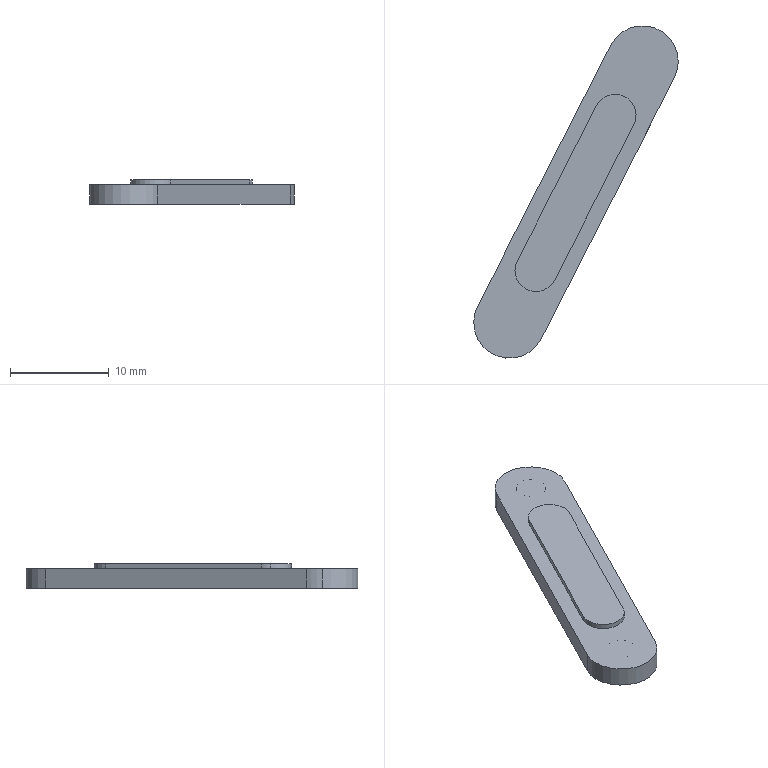Part | SolidWorks | features ICE 3, Extrusion 1 | 1 solid | 19 faces | box 20.758 x 33.747 x 2.5 mm | volume 532.773 mm3 | cylinder 10 | plane 9 | commonest cylinder face diameters 3 x4 4.262 x3 7.265 x3
STEP:
#1=CARTESIAN_POINT('',(1.405,14.797,1.5));
#2=VERTEX_POINT('',#1);
#3=CARTESIAN_POINT('',(5.435,13.83,1.5));
#4=VERTEX_POINT('',#3);
#5=CARTESIAN_POINT('',(3.536,14.797,1.5));
#6=DIRECTION('',(0.,0.,1.));
#7=DIRECTION('',(1.,0.,0.));
#8=AXIS2_PLACEMENT_3D('',#5,#6,#7);
#9=CIRCLE('',#8,2.131);
#10=EDGE_CURVE('',#2,#4,#9,.T.);
#11=ORIENTED_EDGE('',*,*,#10,.F.);
#12=CARTESIAN_POINT('',(1.405,14.797,1.));
#13=VERTEX_POINT('',#12);
#14=CARTESIAN_POINT('',(1.405,14.797,1.5));
#15=DIRECTION('',(0.,0.,-1.));
#16=VECTOR('',#15,1000.);
#17=LINE('',#14,#16);
#18=EDGE_CURVE('',#2,#13,#17,.T.);
#19=ORIENTED_EDGE('',*,*,#18,.T.);
#20=CARTESIAN_POINT('',(5.435,13.83,1.));
#21=VERTEX_POINT('',#20);
#22=CARTESIAN_POINT('',(3.536,14.797,1.));
#23=DIRECTION('',(0.,0.,-1.));
#24=DIRECTION('',(1.,0.,0.));
#25=AXIS2_PLACEMENT_3D('',#22,#23,#24);
#26=CIRCLE('',#25,2.131);
#27=EDGE_CURVE('',#21,#13,#26,.T.);
#28=ORIENTED_EDGE('',*,*,#27,.F.);
#29=CARTESIAN_POINT('',(5.435,13.83,1.5));
#30=DIRECTION('',(0.,0.,-1.));
#31=VECTOR('',#30,1000.);
#32=LINE('',#29,#31);
#33=EDGE_CURVE('',#4,#21,#32,.T.);
#34=ORIENTED_EDGE('',*,*,#33,.F.);
#35=EDGE_LOOP('',(#11,#19,#28,#34));
#36=FACE_OUTER_BOUND('',#35,.T.);
#37=CARTESIAN_POINT('',(3.536,14.797,1.5));
#38=DIRECTION('',(0.,0.,-1.));
#39=DIRECTION('',(-1.,0.,0.));
#40=AXIS2_PLACEMENT_3D('',#37,#38,#39);
#41=CYLINDRICAL_SURFACE('',#40,2.131);
#42=ADVANCED_FACE('',(#36),#41,.T.);
#43=CARTESIAN_POINT('',(-2.775,9.541,1.));
#44=VERTEX_POINT('',#43);
#45=CARTESIAN_POINT('',(4.094,7.891,1.));
#46=VERTEX_POINT('',#45);
#47=CARTESIAN_POINT('',(0.8578,9.541,1.));
#48=DIRECTION('',(0.,0.,1.));
#49=DIRECTION('',(1.,0.,0.));
#50=AXIS2_PLACEMENT_3D('',#47,#48,#49);
#51=CIRCLE('',#50,3.633);
#52=EDGE_CURVE('',#44,#46,#51,.T.);
#53=ORIENTED_EDGE('',*,*,#52,.F.);
#54=CARTESIAN_POINT('',(-2.775,9.541,-1.));
#55=VERTEX_POINT('',#54);
#56=CARTESIAN_POINT('',(-2.775,9.541,1.));
#57=DIRECTION('',(0.,0.,-1.));
#58=VECTOR('',#57,1000.);
#59=LINE('',#56,#58);
#60=EDGE_CURVE('',#44,#55,#59,.T.);
#61=ORIENTED_EDGE('',*,*,#60,.T.);
#62=CARTESIAN_POINT('',(4.094,7.891,-1.));
#63=VERTEX_POINT('',#62);
#64=CARTESIAN_POINT('',(0.8578,9.541,-1.));
#65=DIRECTION('',(0.,0.,1.));
#66=DIRECTION('',(1.,0.,0.));
#67=AXIS2_PLACEMENT_3D('',#64,#65,#66);
#68=CIRCLE('',#67,3.633);
#69=EDGE_CURVE('',#55,#63,#68,.T.);
#70=ORIENTED_EDGE('',*,*,#69,.T.);
#71=CARTESIAN_POINT('',(4.094,7.891,1.));
#72=DIRECTION('',(0.,0.,-1.));
#73=VECTOR('',#72,1000.);
#74=LINE('',#71,#73);
#75=EDGE_CURVE('',#46,#63,#74,.T.);
#76=ORIENTED_EDGE('',*,*,#75,.F.);
#77=EDGE_LOOP('',(#53,#61,#70,#76));
#78=FACE_OUTER_BOUND('',#77,.T.);
#79=CARTESIAN_POINT('',(0.8578,9.541,1.));
#80=DIRECTION('',(0.,0.,-1.));
#81=DIRECTION('',(-1.,0.,0.));
#82=AXIS2_PLACEMENT_3D('',#79,#80,#81);
#83=CYLINDRICAL_SURFACE('',#82,3.633);
#84=ADVANCED_FACE('',(#78),#83,.T.);
#85=CARTESIAN_POINT('',(-0.6422,9.541,0.9));
#86=VERTEX_POINT('',#85);
#87=CARTESIAN_POINT('',(2.358,9.541,0.9));
#88=VERTEX_POINT('',#87);
#89=CARTESIAN_POINT('',(0.8578,9.541,0.9));
#90=DIRECTION('',(0.,0.,1.));
#91=DIRECTION('',(1.,0.,0.));
#92=AXIS2_PLACEMENT_3D('',#89,#90,#91);
#93=CIRCLE('',#92,1.5);
#94=EDGE_CURVE('',#86,#88,#93,.T.);
#95=ORIENTED_EDGE('',*,*,#94,.T.);
#96=CARTESIAN_POINT('',(2.358,9.541,-1.));
#97=VERTEX_POINT('',#96);
#98=CARTESIAN_POINT('',(2.358,9.541,1.));
#99=DIRECTION('',(0.,0.,-1.));
#100=VECTOR('',#99,1000.);
#101=LINE('',#98,#100);
#102=EDGE_CURVE('',#88,#97,#101,.T.);
#103=ORIENTED_EDGE('',*,*,#102,.T.);
#104=CARTESIAN_POINT('',(-0.6422,9.541,-1.));
#105=VERTEX_POINT('',#104);
#106=CARTESIAN_POINT('',(0.8578,9.541,-1.));
#107=DIRECTION('',(0.,0.,1.));
#108=DIRECTION('',(1.,0.,0.));
#109=AXIS2_PLACEMENT_3D('',#106,#107,#108);
#110=CIRCLE('',#109,1.5);
#111=EDGE_CURVE('',#105,#97,#110,.T.);
#112=ORIENTED_EDGE('',*,*,#111,.F.);
#113=CARTESIAN_POINT('',(-0.6422,9.541,1.));
#114=DIRECTION('',(0.,0.,-1.));
#115=VECTOR('',#114,1000.);
#116=LINE('',#113,#115);
#117=EDGE_CURVE('',#86,#105,#116,.T.);
#118=ORIENTED_EDGE('',*,*,#117,.F.);
#119=EDGE_LOOP('',(#95,#103,#112,#118));
#120=FACE_OUTER_BOUND('',#119,.T.);
#121=CARTESIAN_POINT('',(0.8578,9.541,1.));
#122=DIRECTION('',(0.,0.,-1.));
#123=DIRECTION('',(-1.,0.,0.));
#124=AXIS2_PLACEMENT_3D('',#121,#122,#123);
#125=CYLINDRICAL_SURFACE('',#124,1.5);
#126=ADVANCED_FACE('',(#120),#125,.F.);
#127=CARTESIAN_POINT('',(12.851,36.022,0.9));
#128=VERTEX_POINT('',#127);
#129=CARTESIAN_POINT('',(15.851,36.022,0.9));
#130=VERTEX_POINT('',#129);
#131=CARTESIAN_POINT('',(14.351,36.022,0.9));
#132=DIRECTION('',(0.,0.,1.));
#133=DIRECTION('',(1.,0.,0.));
#134=AXIS2_PLACEMENT_3D('',#131,#132,#133);
#135=CIRCLE('',#134,1.5);
#136=EDGE_CURVE('',#128,#130,#135,.T.);
#137=ORIENTED_EDGE('',*,*,#136,.T.);
#138=CARTESIAN_POINT('',(15.851,36.022,-1.));
#139=VERTEX_POINT('',#138);
#140=CARTESIAN_POINT('',(15.851,36.022,1.));
#141=DIRECTION('',(0.,0.,-1.));
#142=VECTOR('',#141,1000.);
#143=LINE('',#140,#142);
#144=EDGE_CURVE('',#130,#139,#143,.T.);
#145=ORIENTED_EDGE('',*,*,#144,.T.);
#146=CARTESIAN_POINT('',(12.851,36.022,-1.));
#147=VERTEX_POINT('',#146);
#148=CARTESIAN_POINT('',(14.351,36.022,-1.));
#149=DIRECTION('',(0.,0.,1.));
#150=DIRECTION('',(1.,0.,0.));
#151=AXIS2_PLACEMENT_3D('',#148,#149,#150);
#152=CIRCLE('',#151,1.5);
#153=EDGE_CURVE('',#147,#139,#152,.T.);
#154=ORIENTED_EDGE('',*,*,#153,.F.);
#155=CARTESIAN_POINT('',(12.851,36.022,1.));
#156=DIRECTION('',(0.,0.,-1.));
#157=VECTOR('',#156,1000.);
#158=LINE('',#155,#157);
#159=EDGE_CURVE('',#128,#147,#158,.T.);
#160=ORIENTED_EDGE('',*,*,#159,.F.);
#161=EDGE_LOOP('',(#137,#145,#154,#160));
#162=FACE_OUTER_BOUND('',#161,.T.);
#163=CARTESIAN_POINT('',(14.351,36.022,1.));
#164=DIRECTION('',(0.,0.,-1.));
#165=DIRECTION('',(-1.,0.,0.));
#166=AXIS2_PLACEMENT_3D('',#163,#164,#165);
#167=CYLINDRICAL_SURFACE('',#166,1.5);
#168=ADVANCED_FACE('',(#162),#167,.F.);
#169=ORIENTED_EDGE('',*,*,#144,.F.);
#170=CARTESIAN_POINT('',(14.351,36.022,0.9));
#171=DIRECTION('',(0.,0.,1.));
#172=DIRECTION('',(1.,0.,0.));
#173=AXIS2_PLACEMENT_3D('',#170,#171,#172);
#174=CIRCLE('',#173,1.5);
#175=EDGE_CURVE('',#130,#128,#174,.T.);
#176=ORIENTED_EDGE('',*,*,#175,.T.);
#177=ORIENTED_EDGE('',*,*,#159,.T.);
#178=CARTESIAN_POINT('',(14.351,36.022,-1.));
#179=DIRECTION('',(0.,0.,1.));
#180=DIRECTION('',(1.,0.,0.));
#181=AXIS2_PLACEMENT_3D('',#178,#179,#180);
#182=CIRCLE('',#181,1.5);
#183=EDGE_CURVE('',#139,#147,#182,.T.);
#184=ORIENTED_EDGE('',*,*,#183,.F.);
#185=EDGE_LOOP('',(#169,#176,#177,#184));
#186=FACE_OUTER_BOUND('',#185,.T.);
#187=CARTESIAN_POINT('',(14.351,36.022,1.));
#188=DIRECTION('',(0.,0.,-1.));
#189=DIRECTION('',(-1.,0.,0.));
#190=AXIS2_PLACEMENT_3D('',#187,#188,#189);
#191=CYLINDRICAL_SURFACE('',#190,1.5);
#192=ADVANCED_FACE('',(#186),#191,.F.);
#193=ORIENTED_EDGE('',*,*,#102,.F.);
#194=CARTESIAN_POINT('',(0.8578,9.541,0.9));
#195=DIRECTION('',(0.,0.,1.));
#196=DIRECTION('',(1.,0.,0.));
#197=AXIS2_PLACEMENT_3D('',#194,#195,#196);
#198=CIRCLE('',#197,1.5);
#199=EDGE_CURVE('',#88,#86,#198,.T.);
#200=ORIENTED_EDGE('',*,*,#199,.T.);
#201=ORIENTED_EDGE('',*,*,#117,.T.);
#202=CARTESIAN_POINT('',(0.8578,9.541,-1.));
#203=DIRECTION('',(0.,0.,1.));
#204=DIRECTION('',(1.,0.,0.));
#205=AXIS2_PLACEMENT_3D('',#202,#203,#204);
#206=CIRCLE('',#205,1.5);
#207=EDGE_CURVE('',#97,#105,#206,.T.);
#208=ORIENTED_EDGE('',*,*,#207,.F.);
#209=EDGE_LOOP('',(#193,#200,#201,#208));
#210=FACE_OUTER_BOUND('',#209,.T.);
#211=CARTESIAN_POINT('',(0.8578,9.541,1.));
#212=DIRECTION('',(0.,0.,-1.));
#213=DIRECTION('',(-1.,0.,0.));
#214=AXIS2_PLACEMENT_3D('',#211,#212,#213);
#215=CYLINDRICAL_SURFACE('',#214,1.5);
#216=ADVANCED_FACE('',(#210),#215,.F.);
#217=CARTESIAN_POINT('',(17.588,34.373,1.));
#218=VERTEX_POINT('',#217);
#219=CARTESIAN_POINT('',(0.05832,-0.02971,1.));
#220=DIRECTION('',(0.454,0.891,0.));
#221=VECTOR('',#220,1000.);
#222=LINE('',#219,#221);
#223=EDGE_CURVE('',#46,#218,#222,.T.);
#224=ORIENTED_EDGE('',*,*,#223,.T.);
#225=CARTESIAN_POINT('',(11.114,37.671,1.));
#226=VERTEX_POINT('',#225);
#227=CARTESIAN_POINT('',(14.351,36.022,1.));
#228=DIRECTION('',(0.,0.,1.));
#229=DIRECTION('',(1.,0.,0.));
#230=AXIS2_PLACEMENT_3D('',#227,#228,#229);
#231=CIRCLE('',#230,3.633);
#232=EDGE_CURVE('',#218,#226,#231,.T.);
#233=ORIENTED_EDGE('',*,*,#232,.T.);
#234=CARTESIAN_POINT('',(-2.379,11.19,1.));
#235=VERTEX_POINT('',#234);
#236=CARTESIAN_POINT('',(-6.415,3.269,1.));
#237=DIRECTION('',(0.454,0.891,0.));
#238=VECTOR('',#237,1000.);
#239=LINE('',#236,#238);
#240=EDGE_CURVE('',#235,#226,#239,.T.);
#241=ORIENTED_EDGE('',*,*,#240,.F.);
#242=CARTESIAN_POINT('',(0.8578,9.541,1.));
#243=DIRECTION('',(0.,0.,1.));
#244=DIRECTION('',(1.,0.,0.));
#245=AXIS2_PLACEMENT_3D('',#242,#243,#244);
#246=CIRCLE('',#245,3.633);
#247=EDGE_CURVE('',#235,#44,#246,.T.);
#248=ORIENTED_EDGE('',*,*,#247,.T.);
#249=ORIENTED_EDGE('',*,*,#52,.T.);
#250=EDGE_LOOP('',(#224,#233,#241,#248,#249));
#251=FACE_OUTER_BOUND('',#250,.T.);
#252=CARTESIAN_POINT('',(13.474,29.607,1.));
#253=VERTEX_POINT('',#252);
#254=CARTESIAN_POINT('',(-1.28,0.652,1.));
#255=DIRECTION('',(-0.454,-0.891,0.));
#256=VECTOR('',#255,1000.);
#257=LINE('',#254,#256);
#258=EDGE_CURVE('',#253,#21,#257,.T.);
#259=ORIENTED_EDGE('',*,*,#258,.T.);
#260=ORIENTED_EDGE('',*,*,#27,.T.);
#261=CARTESIAN_POINT('',(1.637,15.764,1.));
#262=VERTEX_POINT('',#261);
#263=CARTESIAN_POINT('',(3.536,14.797,1.));
#264=DIRECTION('',(0.,0.,-1.));
#265=DIRECTION('',(1.,0.,0.));
#266=AXIS2_PLACEMENT_3D('',#263,#264,#265);
#267=CIRCLE('',#266,2.131);
#268=EDGE_CURVE('',#13,#262,#267,.T.);
#269=ORIENTED_EDGE('',*,*,#268,.T.);
#270=CARTESIAN_POINT('',(9.677,31.542,1.));
#271=VERTEX_POINT('',#270);
#272=CARTESIAN_POINT('',(-5.077,2.587,1.));
#273=DIRECTION('',(0.454,0.891,0.));
#274=VECTOR('',#273,1000.);
#275=LINE('',#272,#274);
#276=EDGE_CURVE('',#262,#271,#275,.T.);
#277=ORIENTED_EDGE('',*,*,#276,.T.);
#278=CARTESIAN_POINT('',(11.575,30.575,1.));
#279=DIRECTION('',(0.,0.,-1.));
#280=DIRECTION('',(1.,0.,0.));
#281=AXIS2_PLACEMENT_3D('',#278,#279,#280);
#282=CIRCLE('',#281,2.131);
#283=EDGE_CURVE('',#271,#253,#282,.T.);
#284=ORIENTED_EDGE('',*,*,#283,.T.);
#285=EDGE_LOOP('',(#259,#260,#269,#277,#284));
#286=FACE_BOUND('',#285,.T.);
#287=CARTESIAN_POINT('',(0.,0.,1.));
#288=DIRECTION('',(0.,0.,1.));
#289=DIRECTION('',(1.,0.,0.));
#290=AXIS2_PLACEMENT_3D('',#287,#288,#289);
#291=PLANE('',#290);
#292=ADVANCED_FACE('',(#251,#286),#291,.T.);
#293=CARTESIAN_POINT('',(17.588,34.373,-1.));
#294=VERTEX_POINT('',#293);
#295=CARTESIAN_POINT('',(0.05832,-0.02971,-1.));
#296=DIRECTION('',(0.454,0.891,0.));
#297=VECTOR('',#296,1000.);
#298=LINE('',#295,#297);
#299=EDGE_CURVE('',#63,#294,#298,.T.);
#300=ORIENTED_EDGE('',*,*,#299,.T.);
#301=CARTESIAN_POINT('',(17.588,34.373,1.));
#302=DIRECTION('',(0.,0.,-1.));
#303=VECTOR('',#302,1000.);
#304=LINE('',#301,#303);
#305=EDGE_CURVE('',#218,#294,#304,.T.);
#306=ORIENTED_EDGE('',*,*,#305,.F.);
#307=ORIENTED_EDGE('',*,*,#223,.F.);
#308=ORIENTED_EDGE('',*,*,#75,.T.);
#309=EDGE_LOOP('',(#300,#306,#307,#308));
#310=FACE_OUTER_BOUND('',#309,.T.);
#311=CARTESIAN_POINT('',(0.05832,-0.02971,1.));
#312=DIRECTION('',(-0.891,0.454,0.));
#313=DIRECTION('',(-0.454,-0.891,0.));
#314=AXIS2_PLACEMENT_3D('',#311,#312,#313);
#315=PLANE('',#314);
#316=ADVANCED_FACE('',(#310),#315,.F.);
#317=CARTESIAN_POINT('',(11.114,37.671,-1.));
#318=VERTEX_POINT('',#317);
#319=CARTESIAN_POINT('',(14.351,36.022,-1.));
#320=DIRECTION('',(0.,0.,1.));
#321=DIRECTION('',(1.,0.,0.));
#322=AXIS2_PLACEMENT_3D('',#319,#320,#321);
#323=CIRCLE('',#322,3.633);
#324=EDGE_CURVE('',#294,#318,#323,.T.);
#325=ORIENTED_EDGE('',*,*,#324,.T.);
#326=CARTESIAN_POINT('',(11.114,37.671,1.));
#327=DIRECTION('',(0.,0.,-1.));
#328=VECTOR('',#327,1000.);
#329=LINE('',#326,#328);
#330=EDGE_CURVE('',#226,#318,#329,.T.);
#331=ORIENTED_EDGE('',*,*,#330,.F.);
#332=ORIENTED_EDGE('',*,*,#232,.F.);
#333=ORIENTED_EDGE('',*,*,#305,.T.);
#334=EDGE_LOOP('',(#325,#331,#332,#333));
#335=FACE_OUTER_BOUND('',#334,.T.);
#336=CARTESIAN_POINT('',(14.351,36.022,1.));
#337=DIRECTION('',(0.,0.,-1.));
#338=DIRECTION('',(-1.,0.,0.));
#339=AXIS2_PLACEMENT_3D('',#336,#337,#338);
#340=CYLINDRICAL_SURFACE('',#339,3.633);
#341=ADVANCED_FACE('',(#335),#340,.T.);
#342=CARTESIAN_POINT('',(-2.379,11.19,-1.));
#343=VERTEX_POINT('',#342);
#344=CARTESIAN_POINT('',(-6.415,3.269,-1.));
#345=DIRECTION('',(0.454,0.891,0.));
#346=VECTOR('',#345,1000.);
#347=LINE('',#344,#346);
#348=EDGE_CURVE('',#343,#318,#347,.T.);
#349=ORIENTED_EDGE('',*,*,#348,.F.);
#350=CARTESIAN_POINT('',(-2.379,11.19,1.));
#351=DIRECTION('',(0.,0.,-1.));
#352=VECTOR('',#351,1000.);
#353=LINE('',#350,#352);
#354=EDGE_CURVE('',#235,#343,#353,.T.);
#355=ORIENTED_EDGE('',*,*,#354,.F.);
#356=ORIENTED_EDGE('',*,*,#240,.T.);
#357=ORIENTED_EDGE('',*,*,#330,.T.);
#358=EDGE_LOOP('',(#349,#355,#356,#357));
#359=FACE_OUTER_BOUND('',#358,.T.);
#360=CARTESIAN_POINT('',(-6.415,3.269,1.));
#361=DIRECTION('',(-0.891,0.454,0.));
#362=DIRECTION('',(-0.454,-0.891,0.));
#363=AXIS2_PLACEMENT_3D('',#360,#361,#362);
#364=PLANE('',#363);
#365=ADVANCED_FACE('',(#359),#364,.T.);
#366=ORIENTED_EDGE('',*,*,#60,.F.);
#367=ORIENTED_EDGE('',*,*,#247,.F.);
#368=ORIENTED_EDGE('',*,*,#354,.T.);
#369=CARTESIAN_POINT('',(0.8578,9.541,-1.));
#370=DIRECTION('',(0.,0.,1.));
#371=DIRECTION('',(1.,0.,0.));
#372=AXIS2_PLACEMENT_3D('',#369,#370,#371);
#373=CIRCLE('',#372,3.633);
#374=EDGE_CURVE('',#343,#55,#373,.T.);
#375=ORIENTED_EDGE('',*,*,#374,.T.);
#376=EDGE_LOOP('',(#366,#367,#368,#375));
#377=FACE_OUTER_BOUND('',#376,.T.);
#378=CARTESIAN_POINT('',(0.8578,9.541,1.));
#379=DIRECTION('',(0.,0.,-1.));
#380=DIRECTION('',(-1.,0.,0.));
#381=AXIS2_PLACEMENT_3D('',#378,#379,#380);
#382=CYLINDRICAL_SURFACE('',#381,3.633);
#383=ADVANCED_FACE('',(#377),#382,.T.);
#384=ORIENTED_EDGE('',*,*,#153,.T.);
#385=ORIENTED_EDGE('',*,*,#183,.T.);
#386=EDGE_LOOP('',(#384,#385));
#387=FACE_BOUND('',#386,.T.);
#388=ORIENTED_EDGE('',*,*,#111,.T.);
#389=ORIENTED_EDGE('',*,*,#207,.T.);
#390=EDGE_LOOP('',(#388,#389));
#391=FACE_BOUND('',#390,.T.);
#392=ORIENTED_EDGE('',*,*,#299,.F.);
#393=ORIENTED_EDGE('',*,*,#69,.F.);
#394=ORIENTED_EDGE('',*,*,#374,.F.);
#395=ORIENTED_EDGE('',*,*,#348,.T.);
#396=ORIENTED_EDGE('',*,*,#324,.F.);
#397=EDGE_LOOP('',(#392,#393,#394,#395,#396));
#398=FACE_OUTER_BOUND('',#397,.T.);
#399=CARTESIAN_POINT('',(0.,0.,-1.));
#400=DIRECTION('',(0.,0.,1.));
#401=DIRECTION('',(1.,0.,0.));
#402=AXIS2_PLACEMENT_3D('',#399,#400,#401);
#403=PLANE('',#402);
#404=ADVANCED_FACE('',(#387,#391,#398),#403,.F.);
#405=ORIENTED_EDGE('',*,*,#18,.F.);
#406=CARTESIAN_POINT('',(1.637,15.764,1.5));
#407=VERTEX_POINT('',#406);
#408=CARTESIAN_POINT('',(3.536,14.797,1.5));
#409=DIRECTION('',(0.,0.,1.));
#410=DIRECTION('',(1.,0.,0.));
#411=AXIS2_PLACEMENT_3D('',#408,#409,#410);
#412=CIRCLE('',#411,2.131);
#413=EDGE_CURVE('',#407,#2,#412,.T.);
#414=ORIENTED_EDGE('',*,*,#413,.F.);
#415=CARTESIAN_POINT('',(1.637,15.764,1.5));
#416=DIRECTION('',(0.,0.,-1.));
#417=VECTOR('',#416,1000.);
#418=LINE('',#415,#417);
#419=EDGE_CURVE('',#407,#262,#418,.T.);
#420=ORIENTED_EDGE('',*,*,#419,.T.);
#421=ORIENTED_EDGE('',*,*,#268,.F.);
#422=EDGE_LOOP('',(#405,#414,#420,#421));
#423=FACE_OUTER_BOUND('',#422,.T.);
#424=CARTESIAN_POINT('',(3.536,14.797,1.5));
#425=DIRECTION('',(0.,0.,-1.));
#426=DIRECTION('',(-1.,0.,0.));
#427=AXIS2_PLACEMENT_3D('',#424,#425,#426);
#428=CYLINDRICAL_SURFACE('',#427,2.131);
#429=ADVANCED_FACE('',(#423),#428,.T.);
#430=ORIENTED_EDGE('',*,*,#258,.F.);
#431=CARTESIAN_POINT('',(13.474,29.607,1.5));
#432=VERTEX_POINT('',#431);
#433=CARTESIAN_POINT('',(13.474,29.607,1.5));
#434=DIRECTION('',(0.,0.,-1.));
#435=VECTOR('',#434,1000.);
#436=LINE('',#433,#435);
#437=EDGE_CURVE('',#432,#253,#436,.T.);
#438=ORIENTED_EDGE('',*,*,#437,.F.);
#439=CARTESIAN_POINT('',(5.435,13.83,1.5));
#440=DIRECTION('',(0.454,0.891,0.));
#441=VECTOR('',#440,1000.);
#442=LINE('',#439,#441);
#443=EDGE_CURVE('',#4,#432,#442,.T.);
#444=ORIENTED_EDGE('',*,*,#443,.F.);
#445=ORIENTED_EDGE('',*,*,#33,.T.);
#446=EDGE_LOOP('',(#430,#438,#444,#445));
#447=FACE_OUTER_BOUND('',#446,.T.);
#448=CARTESIAN_POINT('',(5.435,13.83,1.5));
#449=DIRECTION('',(-0.891,0.454,0.));
#450=DIRECTION('',(-0.454,-0.891,0.));
#451=AXIS2_PLACEMENT_3D('',#448,#449,#450);
#452=PLANE('',#451);
#453=ADVANCED_FACE('',(#447),#452,.F.);
#454=ORIENTED_EDGE('',*,*,#283,.F.);
#455=CARTESIAN_POINT('',(9.677,31.542,1.5));
#456=VERTEX_POINT('',#455);
#457=CARTESIAN_POINT('',(9.677,31.542,1.5));
#458=DIRECTION('',(0.,0.,-1.));
#459=VECTOR('',#458,1000.);
#460=LINE('',#457,#459);
#461=EDGE_CURVE('',#456,#271,#460,.T.);
#462=ORIENTED_EDGE('',*,*,#461,.F.);
#463=CARTESIAN_POINT('',(11.575,30.575,1.5));
#464=DIRECTION('',(0.,0.,1.));
#465=DIRECTION('',(1.,0.,0.));
#466=AXIS2_PLACEMENT_3D('',#463,#464,#465);
#467=CIRCLE('',#466,2.131);
#468=EDGE_CURVE('',#432,#456,#467,.T.);
#469=ORIENTED_EDGE('',*,*,#468,.F.);
#470=ORIENTED_EDGE('',*,*,#437,.T.);
#471=EDGE_LOOP('',(#454,#462,#469,#470));
#472=FACE_OUTER_BOUND('',#471,.T.);
#473=CARTESIAN_POINT('',(11.575,30.575,1.5));
#474=DIRECTION('',(0.,0.,-1.));
#475=DIRECTION('',(-1.,0.,0.));
#476=AXIS2_PLACEMENT_3D('',#473,#474,#475);
#477=CYLINDRICAL_SURFACE('',#476,2.131);
#478=ADVANCED_FACE('',(#472),#477,.T.);
#479=ORIENTED_EDGE('',*,*,#276,.F.);
#480=ORIENTED_EDGE('',*,*,#419,.F.);
#481=CARTESIAN_POINT('',(1.637,15.764,1.5));
#482=DIRECTION('',(-0.454,-0.891,0.));
#483=VECTOR('',#482,1000.);
#484=LINE('',#481,#483);
#485=EDGE_CURVE('',#456,#407,#484,.T.);
#486=ORIENTED_EDGE('',*,*,#485,.F.);
#487=ORIENTED_EDGE('',*,*,#461,.T.);
#488=EDGE_LOOP('',(#479,#480,#486,#487));
#489=FACE_OUTER_BOUND('',#488,.T.);
#490=CARTESIAN_POINT('',(1.637,15.764,1.5));
#491=DIRECTION('',(0.891,-0.454,0.));
#492=DIRECTION('',(0.454,0.891,0.));
#493=AXIS2_PLACEMENT_3D('',#490,#491,#492);
#494=PLANE('',#493);
#495=ADVANCED_FACE('',(#489),#494,.F.);
#496=ORIENTED_EDGE('',*,*,#413,.T.);
#497=ORIENTED_EDGE('',*,*,#10,.T.);
#498=ORIENTED_EDGE('',*,*,#443,.T.);
#499=ORIENTED_EDGE('',*,*,#468,.T.);
#500=ORIENTED_EDGE('',*,*,#485,.T.);
#501=EDGE_LOOP('',(#496,#497,#498,#499,#500));
#502=FACE_OUTER_BOUND('',#501,.T.);
#503=CARTESIAN_POINT('',(3.536,14.797,1.5));
#504=DIRECTION('',(0.,0.,1.));
#505=DIRECTION('',(1.,0.,0.));
#506=AXIS2_PLACEMENT_3D('',#503,#504,#505);
#507=PLANE('',#506);
#508=ADVANCED_FACE('',(#502),#507,.T.);
#509=ORIENTED_EDGE('',*,*,#94,.F.);
#510=ORIENTED_EDGE('',*,*,#199,.F.);
#511=EDGE_LOOP('',(#509,#510));
#512=FACE_OUTER_BOUND('',#511,.T.);
#513=CARTESIAN_POINT('',(0.8578,9.541,0.9));
#514=DIRECTION('',(0.,0.,1.));
#515=DIRECTION('',(1.,0.,0.));
#516=AXIS2_PLACEMENT_3D('',#513,#514,#515);
#517=PLANE('',#516);
#518=ADVANCED_FACE('',(#512),#517,.F.);
#519=ORIENTED_EDGE('',*,*,#136,.F.);
#520=ORIENTED_EDGE('',*,*,#175,.F.);
#521=EDGE_LOOP('',(#519,#520));
#522=FACE_OUTER_BOUND('',#521,.T.);
#523=CARTESIAN_POINT('',(14.351,36.022,0.9));
#524=DIRECTION('',(0.,0.,1.));
#525=DIRECTION('',(1.,0.,0.));
#526=AXIS2_PLACEMENT_3D('',#523,#524,#525);
#527=PLANE('',#526);
#528=ADVANCED_FACE('',(#522),#527,.F.);
#529=CLOSED_SHELL('',(#42,#84,#126,#168,#192,#216,#292,#316,#341,#365,#383,#404,#429,#453,#478,#495,#508,#518,#528));
#530=MANIFOLD_SOLID_BREP('',#529);
#531=CARTESIAN_POINT('',(0.,0.,0.));
#532=DIRECTION('',(0.,0.,1.));
#533=DIRECTION('',(1.,0.,0.));
#534=AXIS2_PLACEMENT_3D('',#531,#532,#533);
#535=(LENGTH_UNIT()NAMED_UNIT(*)SI_UNIT(.MILLI.,.METRE.));
#536=UNCERTAINTY_MEASURE_WITH_UNIT(LENGTH_MEASURE(0.00001),#535,'','');
#537=(NAMED_UNIT(*)PLANE_ANGLE_UNIT()SI_UNIT($,.RADIAN.));
#538=(NAMED_UNIT(*)SI_UNIT($,.STERADIAN.)SOLID_ANGLE_UNIT());
#539=(GEOMETRIC_REPRESENTATION_CONTEXT(3)GLOBAL_UNCERTAINTY_ASSIGNED_CONTEXT((#536))GLOBAL_UNIT_ASSIGNED_CONTEXT((#535,#537,#538))REPRESENTATION_CONTEXT('',''));
#540=ADVANCED_BREP_SHAPE_REPRESENTATION('',(#530,#534),#539);